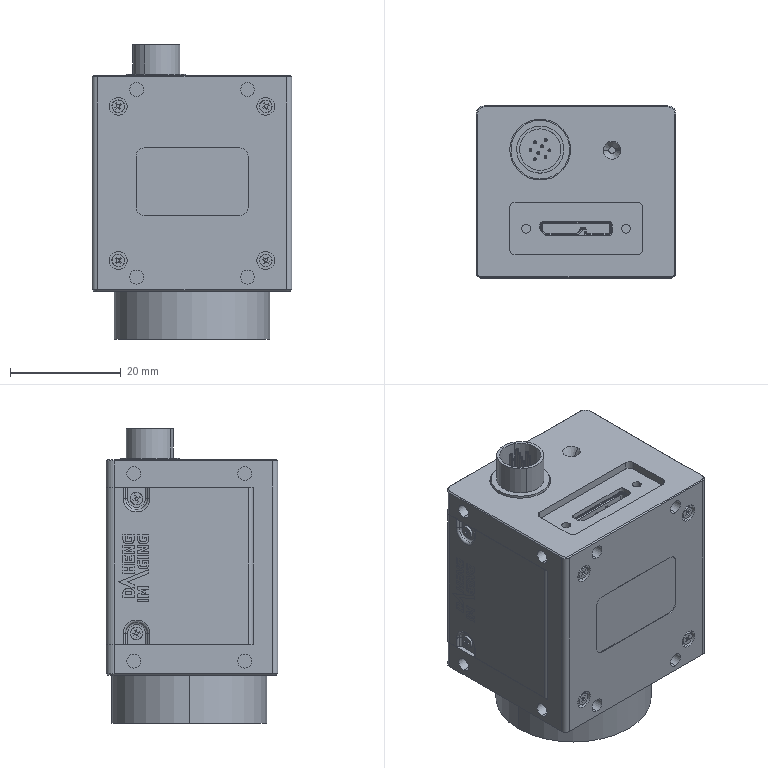Part | SolidWorks | features MBimport 1 | 5 solids | 1218 faces | box 36.008 x 31 x 53.1 mm | volume 39029 mm3 | plane 664 | cylinder 402 | cone 64 | spline 52 | torus 36 | commonest cylinder face diameters 0.4 x42 2 x40 0.8 x32 1.6 x32 2.5 x30 0.3 x29